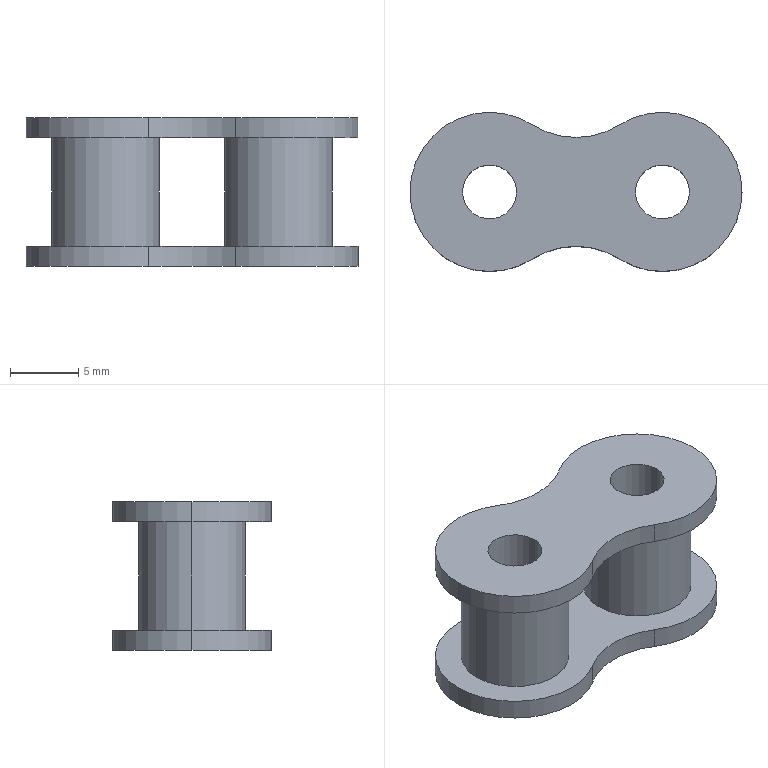Part | STEP file | _CHE40-500_c2 | 1 solid | 24 faces | box 24.4 x 11.7 x 10.95 mm | volume 1210 mm3 | cylinder 20 | plane 4 | commonest cylinder face diameters 11.7 x8 3.97 x4 7.92 x4 11.946 x4
STEP:
#1=CARTESIAN_POINT('',(3.142,4.935,-5.475));
#2=VERTEX_POINT('',#1);
#3=CARTESIAN_POINT('',(9.558,4.935,-5.475));
#4=VERTEX_POINT('',#3);
#5=CARTESIAN_POINT('',(6.35,9.973,-5.475));
#6=DIRECTION('',(0.,0.,1.));
#7=AXIS2_PLACEMENT_3D('',#5,#6,$);
#8=CIRCLE('',#7,5.973);
#9=EDGE_CURVE('',#2,#4,#8,.T.);
#10=ORIENTED_EDGE('',*,*,#9,.T.);
#11=CARTESIAN_POINT('',(18.55,0.,-5.475));
#12=VERTEX_POINT('',#11);
#13=CARTESIAN_POINT('',(12.7,0.,-5.475));
#14=DIRECTION('',(0.,0.,1.));
#15=AXIS2_PLACEMENT_3D('',#13,#14,$);
#16=CIRCLE('',#15,5.85);
#17=EDGE_CURVE('',#12,#4,#16,.T.);
#18=ORIENTED_EDGE('',*,*,#17,.F.);
#19=CARTESIAN_POINT('',(9.558,-4.935,-5.475));
#20=VERTEX_POINT('',#19);
#21=CARTESIAN_POINT('',(12.7,0.,-5.475));
#22=DIRECTION('',(0.,0.,1.));
#23=AXIS2_PLACEMENT_3D('',#21,#22,$);
#24=CIRCLE('',#23,5.85);
#25=EDGE_CURVE('',#20,#12,#24,.T.);
#26=ORIENTED_EDGE('',*,*,#25,.F.);
#27=CARTESIAN_POINT('',(3.142,-4.935,-5.475));
#28=VERTEX_POINT('',#27);
#29=CARTESIAN_POINT('',(6.35,-9.973,-5.475));
#30=DIRECTION('',(0.,0.,1.));
#31=AXIS2_PLACEMENT_3D('',#29,#30,$);
#32=CIRCLE('',#31,5.973);
#33=EDGE_CURVE('',#20,#28,#32,.T.);
#34=ORIENTED_EDGE('',*,*,#33,.T.);
#35=CARTESIAN_POINT('',(-5.85,0.,-5.475));
#36=VERTEX_POINT('',#35);
#37=CARTESIAN_POINT('',(0.,-0.000000001,-5.475));
#38=DIRECTION('',(0.,0.,1.));
#39=AXIS2_PLACEMENT_3D('',#37,#38,$);
#40=CIRCLE('',#39,5.85);
#41=EDGE_CURVE('',#36,#28,#40,.T.);
#42=ORIENTED_EDGE('',*,*,#41,.F.);
#43=CARTESIAN_POINT('',(0.,-0.000000001,-5.475));
#44=DIRECTION('',(0.,0.,1.));
#45=AXIS2_PLACEMENT_3D('',#43,#44,$);
#46=CIRCLE('',#45,5.85);
#47=EDGE_CURVE('',#2,#36,#46,.T.);
#48=ORIENTED_EDGE('',*,*,#47,.F.);
#49=EDGE_LOOP('',(#10,#18,#26,#34,#42,#48));
#50=FACE_OUTER_BOUND('',#49,.T.);
#51=CARTESIAN_POINT('',(10.715,0.000000001,-5.475));
#52=VERTEX_POINT('',#51);
#53=CARTESIAN_POINT('',(14.685,0.000000001,-5.475));
#54=VERTEX_POINT('',#53);
#55=CARTESIAN_POINT('',(12.7,0.,-5.475));
#56=DIRECTION('',(0.,0.,1.));
#57=AXIS2_PLACEMENT_3D('',#55,#56,$);
#58=CIRCLE('',#57,1.985);
#59=EDGE_CURVE('',#52,#54,#58,.F.);
#60=ORIENTED_EDGE('',*,*,#59,.F.);
#61=CARTESIAN_POINT('',(12.7,0.,-5.475));
#62=DIRECTION('',(0.,0.,1.));
#63=AXIS2_PLACEMENT_3D('',#61,#62,$);
#64=CIRCLE('',#63,1.985);
#65=EDGE_CURVE('',#54,#52,#64,.F.);
#66=ORIENTED_EDGE('',*,*,#65,.F.);
#67=EDGE_LOOP('',(#60,#66));
#68=FACE_BOUND('',#67,.T.);
#69=CARTESIAN_POINT('',(-1.985,0.000000001,-5.475));
#70=VERTEX_POINT('',#69);
#71=CARTESIAN_POINT('',(1.985,0.000000001,-5.475));
#72=VERTEX_POINT('',#71);
#73=CARTESIAN_POINT('',(0.000000001,0.,-5.475));
#74=DIRECTION('',(0.,0.,1.));
#75=AXIS2_PLACEMENT_3D('',#73,#74,$);
#76=CIRCLE('',#75,1.985);
#77=EDGE_CURVE('',#70,#72,#76,.F.);
#78=ORIENTED_EDGE('',*,*,#77,.F.);
#79=CARTESIAN_POINT('',(0.000000001,0.,-5.475));
#80=DIRECTION('',(0.,0.,1.));
#81=AXIS2_PLACEMENT_3D('',#79,#80,$);
#82=CIRCLE('',#81,1.985);
#83=EDGE_CURVE('',#72,#70,#82,.F.);
#84=ORIENTED_EDGE('',*,*,#83,.F.);
#85=EDGE_LOOP('',(#78,#84));
#86=FACE_BOUND('',#85,.T.);
#87=CARTESIAN_POINT('',(9.525,4.986,-5.475));
#88=DIRECTION('',(0.,0.,1.));
#89=DIRECTION('',(1.,0.,0.));
#90=AXIS2_PLACEMENT_3D('',#87,#88,#89);
#91=PLANE('',#90);
#92=ADVANCED_FACE('',(#50,#68,#86),#91,.F.);
#93=CARTESIAN_POINT('',(3.142,4.935,-3.975));
#94=VERTEX_POINT('',#93);
#95=CARTESIAN_POINT('',(9.558,4.935,-3.975));
#96=VERTEX_POINT('',#95);
#97=CARTESIAN_POINT('',(6.35,9.973,-3.975));
#98=DIRECTION('',(0.,0.,-1.));
#99=AXIS2_PLACEMENT_3D('',#97,#98,$);
#100=CIRCLE('',#99,5.973);
#101=EDGE_CURVE('',#94,#96,#100,.F.);
#102=ORIENTED_EDGE('',*,*,#101,.T.);
#103=CARTESIAN_POINT('',(9.558,4.935,-5.475));
#104=DIRECTION('',(0.,0.,-1.));
#105=VECTOR('',#104,1.);
#106=LINE('',#103,#105);
#107=EDGE_CURVE('',#4,#96,#106,.F.);
#108=ORIENTED_EDGE('',*,*,#107,.F.);
#109=ORIENTED_EDGE('',*,*,#9,.F.);
#110=CARTESIAN_POINT('',(3.142,4.935,-5.475));
#111=DIRECTION('',(0.,0.,-1.));
#112=VECTOR('',#111,1.);
#113=LINE('',#110,#112);
#114=EDGE_CURVE('',#2,#94,#113,.F.);
#115=ORIENTED_EDGE('',*,*,#114,.T.);
#116=EDGE_LOOP('',(#102,#108,#109,#115));
#117=FACE_OUTER_BOUND('',#116,.T.);
#118=CARTESIAN_POINT('',(6.35,9.973,-5.475));
#119=DIRECTION('',(0.,0.,-1.));
#120=DIRECTION('',(1.,0.,0.));
#121=AXIS2_PLACEMENT_3D('',#118,#119,#120);
#122=CYLINDRICAL_SURFACE('',#121,5.973);
#123=ADVANCED_FACE('',(#117),#122,.F.);
#124=CARTESIAN_POINT('',(18.55,0.,-3.975));
#125=VERTEX_POINT('',#124);
#126=CARTESIAN_POINT('',(18.55,0.,-5.475));
#127=DIRECTION('',(0.,0.,-1.));
#128=VECTOR('',#127,1.);
#129=LINE('',#126,#128);
#130=EDGE_CURVE('',#12,#125,#129,.F.);
#131=ORIENTED_EDGE('',*,*,#130,.F.);
#132=ORIENTED_EDGE('',*,*,#17,.T.);
#133=ORIENTED_EDGE('',*,*,#107,.T.);
#134=CARTESIAN_POINT('',(12.7,0.,-3.975));
#135=DIRECTION('',(0.,0.,-1.));
#136=AXIS2_PLACEMENT_3D('',#134,#135,$);
#137=CIRCLE('',#136,5.85);
#138=EDGE_CURVE('',#125,#96,#137,.F.);
#139=ORIENTED_EDGE('',*,*,#138,.F.);
#140=EDGE_LOOP('',(#131,#132,#133,#139));
#141=FACE_OUTER_BOUND('',#140,.T.);
#142=CARTESIAN_POINT('',(12.7,0.,-5.475));
#143=DIRECTION('',(0.,0.,-1.));
#144=DIRECTION('',(-1.,0.,0.));
#145=AXIS2_PLACEMENT_3D('',#142,#143,#144);
#146=CYLINDRICAL_SURFACE('',#145,5.85);
#147=ADVANCED_FACE('',(#141),#146,.T.);
#148=ORIENTED_EDGE('',*,*,#130,.T.);
#149=CARTESIAN_POINT('',(9.558,-4.935,-3.975));
#150=VERTEX_POINT('',#149);
#151=CARTESIAN_POINT('',(12.7,0.,-3.975));
#152=DIRECTION('',(0.,0.,-1.));
#153=AXIS2_PLACEMENT_3D('',#151,#152,$);
#154=CIRCLE('',#153,5.85);
#155=EDGE_CURVE('',#150,#125,#154,.F.);
#156=ORIENTED_EDGE('',*,*,#155,.F.);
#157=CARTESIAN_POINT('',(9.558,-4.935,-5.475));
#158=DIRECTION('',(0.,0.,-1.));
#159=VECTOR('',#158,1.);
#160=LINE('',#157,#159);
#161=EDGE_CURVE('',#20,#150,#160,.F.);
#162=ORIENTED_EDGE('',*,*,#161,.F.);
#163=ORIENTED_EDGE('',*,*,#25,.T.);
#164=EDGE_LOOP('',(#148,#156,#162,#163));
#165=FACE_OUTER_BOUND('',#164,.T.);
#166=CARTESIAN_POINT('',(12.7,0.,-5.475));
#167=DIRECTION('',(0.,0.,-1.));
#168=DIRECTION('',(1.,0.,0.));
#169=AXIS2_PLACEMENT_3D('',#166,#167,#168);
#170=CYLINDRICAL_SURFACE('',#169,5.85);
#171=ADVANCED_FACE('',(#165),#170,.T.);
#172=CARTESIAN_POINT('',(3.142,-4.935,-3.975));
#173=VERTEX_POINT('',#172);
#174=CARTESIAN_POINT('',(6.35,-9.973,-3.975));
#175=DIRECTION('',(0.,0.,-1.));
#176=AXIS2_PLACEMENT_3D('',#174,#175,$);
#177=CIRCLE('',#176,5.973);
#178=EDGE_CURVE('',#150,#173,#177,.F.);
#179=ORIENTED_EDGE('',*,*,#178,.T.);
#180=CARTESIAN_POINT('',(3.142,-4.935,-5.475));
#181=DIRECTION('',(0.,0.,-1.));
#182=VECTOR('',#181,1.);
#183=LINE('',#180,#182);
#184=EDGE_CURVE('',#28,#173,#183,.F.);
#185=ORIENTED_EDGE('',*,*,#184,.F.);
#186=ORIENTED_EDGE('',*,*,#33,.F.);
#187=ORIENTED_EDGE('',*,*,#161,.T.);
#188=EDGE_LOOP('',(#179,#185,#186,#187));
#189=FACE_OUTER_BOUND('',#188,.T.);
#190=CARTESIAN_POINT('',(6.35,-9.973,-5.475));
#191=DIRECTION('',(0.,0.,-1.));
#192=DIRECTION('',(-1.,0.,0.));
#193=AXIS2_PLACEMENT_3D('',#190,#191,#192);
#194=CYLINDRICAL_SURFACE('',#193,5.973);
#195=ADVANCED_FACE('',(#189),#194,.F.);
#196=CARTESIAN_POINT('',(-5.85,0.,-3.975));
#197=VERTEX_POINT('',#196);
#198=CARTESIAN_POINT('',(-5.85,0.,-5.475));
#199=DIRECTION('',(0.,0.,-1.));
#200=VECTOR('',#199,1.);
#201=LINE('',#198,#200);
#202=EDGE_CURVE('',#197,#36,#201,.T.);
#203=ORIENTED_EDGE('',*,*,#202,.T.);
#204=ORIENTED_EDGE('',*,*,#41,.T.);
#205=ORIENTED_EDGE('',*,*,#184,.T.);
#206=CARTESIAN_POINT('',(0.,0.,-3.975));
#207=DIRECTION('',(0.,0.,-1.));
#208=AXIS2_PLACEMENT_3D('',#206,#207,$);
#209=CIRCLE('',#208,5.85);
#210=EDGE_CURVE('',#197,#173,#209,.F.);
#211=ORIENTED_EDGE('',*,*,#210,.F.);
#212=EDGE_LOOP('',(#203,#204,#205,#211));
#213=FACE_OUTER_BOUND('',#212,.T.);
#214=CARTESIAN_POINT('',(0.,0.,-5.475));
#215=DIRECTION('',(0.,0.,-1.));
#216=DIRECTION('',(1.,0.,0.));
#217=AXIS2_PLACEMENT_3D('',#214,#215,#216);
#218=CYLINDRICAL_SURFACE('',#217,5.85);
#219=ADVANCED_FACE('',(#213),#218,.T.);
#220=ORIENTED_EDGE('',*,*,#202,.F.);
#221=CARTESIAN_POINT('',(0.,0.,-3.975));
#222=DIRECTION('',(0.,0.,-1.));
#223=AXIS2_PLACEMENT_3D('',#221,#222,$);
#224=CIRCLE('',#223,5.85);
#225=EDGE_CURVE('',#94,#197,#224,.F.);
#226=ORIENTED_EDGE('',*,*,#225,.F.);
#227=ORIENTED_EDGE('',*,*,#114,.F.);
#228=ORIENTED_EDGE('',*,*,#47,.T.);
#229=EDGE_LOOP('',(#220,#226,#227,#228));
#230=FACE_OUTER_BOUND('',#229,.T.);
#231=CARTESIAN_POINT('',(0.,0.,-5.475));
#232=DIRECTION('',(0.,0.,-1.));
#233=DIRECTION('',(-1.,0.,0.));
#234=AXIS2_PLACEMENT_3D('',#231,#232,#233);
#235=CYLINDRICAL_SURFACE('',#234,5.85);
#236=ADVANCED_FACE('',(#230),#235,.T.);
#237=CARTESIAN_POINT('',(10.715,0.000000001,5.475));
#238=VERTEX_POINT('',#237);
#239=CARTESIAN_POINT('',(14.685,0.000000001,5.475));
#240=VERTEX_POINT('',#239);
#241=CARTESIAN_POINT('',(12.7,0.,5.475));
#242=DIRECTION('',(0.,0.,-1.));
#243=AXIS2_PLACEMENT_3D('',#241,#242,$);
#244=CIRCLE('',#243,1.985);
#245=EDGE_CURVE('',#238,#240,#244,.T.);
#246=ORIENTED_EDGE('',*,*,#245,.F.);
#247=CARTESIAN_POINT('',(10.715,0.,6.975));
#248=DIRECTION('',(0.,0.,-1.));
#249=VECTOR('',#248,1.);
#250=LINE('',#247,#249);
#251=EDGE_CURVE('',#238,#52,#250,.T.);
#252=ORIENTED_EDGE('',*,*,#251,.T.);
#253=ORIENTED_EDGE('',*,*,#59,.T.);
#254=CARTESIAN_POINT('',(14.685,0.,6.975));
#255=DIRECTION('',(0.,0.,-1.));
#256=VECTOR('',#255,1.);
#257=LINE('',#254,#256);
#258=EDGE_CURVE('',#54,#240,#257,.F.);
#259=ORIENTED_EDGE('',*,*,#258,.T.);
#260=EDGE_LOOP('',(#246,#252,#253,#259));
#261=FACE_OUTER_BOUND('',#260,.T.);
#262=CARTESIAN_POINT('',(12.7,0.,6.975));
#263=DIRECTION('',(0.,0.,-1.));
#264=DIRECTION('',(-1.,0.,0.));
#265=AXIS2_PLACEMENT_3D('',#262,#263,#264);
#266=CYLINDRICAL_SURFACE('',#265,1.985);
#267=ADVANCED_FACE('',(#261),#266,.F.);
#268=CARTESIAN_POINT('',(12.7,0.,5.475));
#269=DIRECTION('',(0.,0.,-1.));
#270=AXIS2_PLACEMENT_3D('',#268,#269,$);
#271=CIRCLE('',#270,1.985);
#272=EDGE_CURVE('',#240,#238,#271,.T.);
#273=ORIENTED_EDGE('',*,*,#272,.F.);
#274=ORIENTED_EDGE('',*,*,#258,.F.);
#275=ORIENTED_EDGE('',*,*,#65,.T.);
#276=ORIENTED_EDGE('',*,*,#251,.F.);
#277=EDGE_LOOP('',(#273,#274,#275,#276));
#278=FACE_OUTER_BOUND('',#277,.T.);
#279=CARTESIAN_POINT('',(12.7,0.,6.975));
#280=DIRECTION('',(0.,0.,-1.));
#281=DIRECTION('',(1.,0.,0.));
#282=AXIS2_PLACEMENT_3D('',#279,#280,#281);
#283=CYLINDRICAL_SURFACE('',#282,1.985);
#284=ADVANCED_FACE('',(#278),#283,.F.);
#285=CARTESIAN_POINT('',(-1.985,0.000000001,5.475));
#286=VERTEX_POINT('',#285);
#287=CARTESIAN_POINT('',(1.985,0.000000001,5.475));
#288=VERTEX_POINT('',#287);
#289=CARTESIAN_POINT('',(0.,0.,5.475));
#290=DIRECTION('',(0.,0.,-1.));
#291=AXIS2_PLACEMENT_3D('',#289,#290,$);
#292=CIRCLE('',#291,1.985);
#293=EDGE_CURVE('',#286,#288,#292,.T.);
#294=ORIENTED_EDGE('',*,*,#293,.F.);
#295=CARTESIAN_POINT('',(-1.985,0.,6.975));
#296=DIRECTION('',(0.,0.,-1.));
#297=VECTOR('',#296,1.);
#298=LINE('',#295,#297);
#299=EDGE_CURVE('',#286,#70,#298,.T.);
#300=ORIENTED_EDGE('',*,*,#299,.T.);
#301=ORIENTED_EDGE('',*,*,#77,.T.);
#302=CARTESIAN_POINT('',(1.985,0.,6.975));
#303=DIRECTION('',(0.,0.,-1.));
#304=VECTOR('',#303,1.);
#305=LINE('',#302,#304);
#306=EDGE_CURVE('',#72,#288,#305,.F.);
#307=ORIENTED_EDGE('',*,*,#306,.T.);
#308=EDGE_LOOP('',(#294,#300,#301,#307));
#309=FACE_OUTER_BOUND('',#308,.T.);
#310=CARTESIAN_POINT('',(0.,0.,6.975));
#311=DIRECTION('',(0.,0.,-1.));
#312=DIRECTION('',(-1.,0.,0.));
#313=AXIS2_PLACEMENT_3D('',#310,#311,#312);
#314=CYLINDRICAL_SURFACE('',#313,1.985);
#315=ADVANCED_FACE('',(#309),#314,.F.);
#316=CARTESIAN_POINT('',(0.,0.,5.475));
#317=DIRECTION('',(0.,0.,-1.));
#318=AXIS2_PLACEMENT_3D('',#316,#317,$);
#319=CIRCLE('',#318,1.985);
#320=EDGE_CURVE('',#288,#286,#319,.T.);
#321=ORIENTED_EDGE('',*,*,#320,.F.);
#322=ORIENTED_EDGE('',*,*,#306,.F.);
#323=ORIENTED_EDGE('',*,*,#83,.T.);
#324=ORIENTED_EDGE('',*,*,#299,.F.);
#325=EDGE_LOOP('',(#321,#322,#323,#324));
#326=FACE_OUTER_BOUND('',#325,.T.);
#327=CARTESIAN_POINT('',(0.,0.,6.975));
#328=DIRECTION('',(0.,0.,-1.));
#329=DIRECTION('',(1.,0.,0.));
#330=AXIS2_PLACEMENT_3D('',#327,#328,#329);
#331=CYLINDRICAL_SURFACE('',#330,1.985);
#332=ADVANCED_FACE('',(#326),#331,.F.);
#333=ORIENTED_EDGE('',*,*,#101,.F.);
#334=ORIENTED_EDGE('',*,*,#225,.T.);
#335=ORIENTED_EDGE('',*,*,#210,.T.);
#336=ORIENTED_EDGE('',*,*,#178,.F.);
#337=ORIENTED_EDGE('',*,*,#155,.T.);
#338=ORIENTED_EDGE('',*,*,#138,.T.);
#339=EDGE_LOOP('',(#333,#334,#335,#336,#337,#338));
#340=FACE_OUTER_BOUND('',#339,.T.);
#341=CARTESIAN_POINT('',(-3.96,0.000000001,-3.975));
#342=VERTEX_POINT('',#341);
#343=CARTESIAN_POINT('',(3.96,0.000000001,-3.975));
#344=VERTEX_POINT('',#343);
#345=CARTESIAN_POINT('',(0.000000001,0.,-3.975));
#346=DIRECTION('',(0.,0.,1.));
#347=AXIS2_PLACEMENT_3D('',#345,#346,$);
#348=CIRCLE('',#347,3.96);
#349=EDGE_CURVE('',#342,#344,#348,.T.);
#350=ORIENTED_EDGE('',*,*,#349,.F.);
#351=CARTESIAN_POINT('',(0.000000001,0.,-3.975));
#352=DIRECTION('',(0.,0.,1.));
#353=AXIS2_PLACEMENT_3D('',#351,#352,$);
#354=CIRCLE('',#353,3.96);
#355=EDGE_CURVE('',#344,#342,#354,.T.);
#356=ORIENTED_EDGE('',*,*,#355,.F.);
#357=EDGE_LOOP('',(#350,#356));
#358=FACE_BOUND('',#357,.T.);
#359=CARTESIAN_POINT('',(8.74,0.000000001,-3.975));
#360=VERTEX_POINT('',#359);
#361=CARTESIAN_POINT('',(16.66,0.000000001,-3.975));
#362=VERTEX_POINT('',#361);
#363=CARTESIAN_POINT('',(12.7,0.,-3.975));
#364=DIRECTION('',(0.,0.,1.));
#365=AXIS2_PLACEMENT_3D('',#363,#364,$);
#366=CIRCLE('',#365,3.96);
#367=EDGE_CURVE('',#360,#362,#366,.T.);
#368=ORIENTED_EDGE('',*,*,#367,.F.);
#369=CARTESIAN_POINT('',(12.7,0.,-3.975));
#370=DIRECTION('',(0.,0.,1.));
#371=AXIS2_PLACEMENT_3D('',#369,#370,$);
#372=CIRCLE('',#371,3.96);
#373=EDGE_CURVE('',#362,#360,#372,.T.);
#374=ORIENTED_EDGE('',*,*,#373,.F.);
#375=EDGE_LOOP('',(#368,#374));
#376=FACE_BOUND('',#375,.T.);
#377=CARTESIAN_POINT('',(9.525,4.986,-3.975));
#378=DIRECTION('',(0.,0.,1.));
#379=DIRECTION('',(1.,0.,0.));
#380=AXIS2_PLACEMENT_3D('',#377,#378,#379);
#381=PLANE('',#380);
#382=ADVANCED_FACE('',(#340,#358,#376),#381,.T.);
#383=CARTESIAN_POINT('',(3.142,4.935,5.475));
#384=VERTEX_POINT('',#383);
#385=CARTESIAN_POINT('',(9.558,4.935,5.475));
#386=VERTEX_POINT('',#385);
#387=CARTESIAN_POINT('',(6.35,9.973,5.475));
#388=DIRECTION('',(0.,0.,1.));
#389=AXIS2_PLACEMENT_3D('',#387,#388,$);
#390=CIRCLE('',#389,5.973);
#391=EDGE_CURVE('',#384,#386,#390,.T.);
#392=ORIENTED_EDGE('',*,*,#391,.F.);
#393=CARTESIAN_POINT('',(-5.85,0.,5.475));
#394=VERTEX_POINT('',#393);
#395=CARTESIAN_POINT('',(0.,-0.000000001,5.475));
#396=DIRECTION('',(0.,0.,1.));
#397=AXIS2_PLACEMENT_3D('',#395,#396,$);
#398=CIRCLE('',#397,5.85);
#399=EDGE_CURVE('',#384,#394,#398,.T.);
#400=ORIENTED_EDGE('',*,*,#399,.T.);
#401=CARTESIAN_POINT('',(3.142,-4.935,5.475));
#402=VERTEX_POINT('',#401);
#403=CARTESIAN_POINT('',(0.,-0.000000001,5.475));
#404=DIRECTION('',(0.,0.,1.));
#405=AXIS2_PLACEMENT_3D('',#403,#404,$);
#406=CIRCLE('',#405,5.85);
#407=EDGE_CURVE('',#394,#402,#406,.T.);
#408=ORIENTED_EDGE('',*,*,#407,.T.);
#409=CARTESIAN_POINT('',(9.558,-4.935,5.475));
#410=VERTEX_POINT('',#409);
#411=CARTESIAN_POINT('',(6.35,-9.973,5.475));
#412=DIRECTION('',(0.,0.,1.));
#413=AXIS2_PLACEMENT_3D('',#411,#412,$);
#414=CIRCLE('',#413,5.973);
#415=EDGE_CURVE('',#410,#402,#414,.T.);
#416=ORIENTED_EDGE('',*,*,#415,.F.);
#417=CARTESIAN_POINT('',(18.55,0.,5.475));
#418=VERTEX_POINT('',#417);
#419=CARTESIAN_POINT('',(12.7,0.,5.475));
#420=DIRECTION('',(0.,0.,1.));
#421=AXIS2_PLACEMENT_3D('',#419,#420,$);
#422=CIRCLE('',#421,5.85);
#423=EDGE_CURVE('',#410,#418,#422,.T.);
#424=ORIENTED_EDGE('',*,*,#423,.T.);
#425=CARTESIAN_POINT('',(12.7,0.,5.475));
#426=DIRECTION('',(0.,0.,1.));
#427=AXIS2_PLACEMENT_3D('',#425,#426,$);
#428=CIRCLE('',#427,5.85);
#429=EDGE_CURVE('',#418,#386,#428,.T.);
#430=ORIENTED_EDGE('',*,*,#429,.T.);
#431=EDGE_LOOP('',(#392,#400,#408,#416,#424,#430));
#432=FACE_OUTER_BOUND('',#431,.T.);
#433=ORIENTED_EDGE('',*,*,#272,.T.);
#434=ORIENTED_EDGE('',*,*,#245,.T.);
#435=EDGE_LOOP('',(#433,#434));
#436=FACE_BOUND('',#435,.T.);
#437=ORIENTED_EDGE('',*,*,#320,.T.);
#438=ORIENTED_EDGE('',*,*,#293,.T.);
#439=EDGE_LOOP('',(#437,#438));
#440=FACE_BOUND('',#439,.T.);
#441=CARTESIAN_POINT('',(9.525,4.986,5.475));
#442=DIRECTION('',(0.,0.,1.));
#443=DIRECTION('',(1.,0.,0.));
#444=AXIS2_PLACEMENT_3D('',#441,#442,#443);
#445=PLANE('',#444);
#446=ADVANCED_FACE('',(#432,#436,#440),#445,.T.);
#447=CARTESIAN_POINT('',(-3.96,0.000000001,3.975));
#448=VERTEX_POINT('',#447);
#449=CARTESIAN_POINT('',(-3.96,0.,4.725));
#450=DIRECTION('',(0.,0.,-1.));
#451=VECTOR('',#450,1.);
#452=LINE('',#449,#451);
#453=EDGE_CURVE('',#448,#342,#452,.T.);
#454=ORIENTED_EDGE('',*,*,#453,.T.);
#455=ORIENTED_EDGE('',*,*,#349,.T.);
#456=CARTESIAN_POINT('',(3.96,0.000000001,3.975));
#457=VERTEX_POINT('',#456);
#458=CARTESIAN_POINT('',(3.96,0.,4.725));
#459=DIRECTION('',(0.,0.,-1.));
#460=VECTOR('',#459,1.);
#461=LINE('',#458,#460);
#462=EDGE_CURVE('',#344,#457,#461,.F.);
#463=ORIENTED_EDGE('',*,*,#462,.T.);
#464=CARTESIAN_POINT('',(0.,0.,3.975));
#465=DIRECTION('',(0.,0.,-1.));
#466=AXIS2_PLACEMENT_3D('',#464,#465,$);
#467=CIRCLE('',#466,3.96);
#468=EDGE_CURVE('',#457,#448,#467,.T.);
#469=ORIENTED_EDGE('',*,*,#468,.T.);
#470=EDGE_LOOP('',(#454,#455,#463,#469));
#471=FACE_OUTER_BOUND('',#470,.T.);
#472=CARTESIAN_POINT('',(0.,0.,4.725));
#473=DIRECTION('',(0.,0.,-1.));
#474=DIRECTION('',(1.,0.,0.));
#475=AXIS2_PLACEMENT_3D('',#472,#473,#474);
#476=CYLINDRICAL_SURFACE('',#475,3.96);
#477=ADVANCED_FACE('',(#471),#476,.T.);
#478=ORIENTED_EDGE('',*,*,#462,.F.);
#479=ORIENTED_EDGE('',*,*,#355,.T.);
#480=ORIENTED_EDGE('',*,*,#453,.F.);
#481=CARTESIAN_POINT('',(0.,0.,3.975));
#482=DIRECTION('',(0.,0.,-1.));
#483=AXIS2_PLACEMENT_3D('',#481,#482,$);
#484=CIRCLE('',#483,3.96);
#485=EDGE_CURVE('',#448,#457,#484,.T.);
#486=ORIENTED_EDGE('',*,*,#485,.T.);
#487=EDGE_LOOP('',(#478,#479,#480,#486));
#488=FACE_OUTER_BOUND('',#487,.T.);
#489=CARTESIAN_POINT('',(0.,0.,4.725));
#490=DIRECTION('',(0.,0.,-1.));
#491=DIRECTION('',(-1.,0.,0.));
#492=AXIS2_PLACEMENT_3D('',#489,#490,#491);
#493=CYLINDRICAL_SURFACE('',#492,3.96);
#494=ADVANCED_FACE('',(#488),#493,.T.);
#495=CARTESIAN_POINT('',(8.74,0.000000001,3.975));
#496=VERTEX_POINT('',#495);
#497=CARTESIAN_POINT('',(8.74,0.,4.725));
#498=DIRECTION('',(0.,0.,-1.));
#499=VECTOR('',#498,1.);
#500=LINE('',#497,#499);
#501=EDGE_CURVE('',#496,#360,#500,.T.);
#502=ORIENTED_EDGE('',*,*,#501,.T.);
#503=ORIENTED_EDGE('',*,*,#367,.T.);
#504=CARTESIAN_POINT('',(16.66,0.000000001,3.975));
#505=VERTEX_POINT('',#504);
#506=CARTESIAN_POINT('',(16.66,0.,4.725));
#507=DIRECTION('',(0.,0.,-1.));
#508=VECTOR('',#507,1.);
#509=LINE('',#506,#508);
#510=EDGE_CURVE('',#362,#505,#509,.F.);
#511=ORIENTED_EDGE('',*,*,#510,.T.);
#512=CARTESIAN_POINT('',(12.7,0.,3.975));
#513=DIRECTION('',(0.,0.,-1.));
#514=AXIS2_PLACEMENT_3D('',#512,#513,$);
#515=CIRCLE('',#514,3.96);
#516=EDGE_CURVE('',#505,#496,#515,.T.);
#517=ORIENTED_EDGE('',*,*,#516,.T.);
#518=EDGE_LOOP('',(#502,#503,#511,#517));
#519=FACE_OUTER_BOUND('',#518,.T.);
#520=CARTESIAN_POINT('',(12.7,0.,4.725));
#521=DIRECTION('',(0.,0.,-1.));
#522=DIRECTION('',(1.,0.,0.));
#523=AXIS2_PLACEMENT_3D('',#520,#521,#522);
#524=CYLINDRICAL_SURFACE('',#523,3.96);
#525=ADVANCED_FACE('',(#519),#524,.T.);
#526=ORIENTED_EDGE('',*,*,#510,.F.);
#527=ORIENTED_EDGE('',*,*,#373,.T.);
#528=ORIENTED_EDGE('',*,*,#501,.F.);
#529=CARTESIAN_POINT('',(12.7,0.,3.975));
#530=DIRECTION('',(0.,0.,-1.));
#531=AXIS2_PLACEMENT_3D('',#529,#530,$);
#532=CIRCLE('',#531,3.96);
#533=EDGE_CURVE('',#496,#505,#532,.T.);
#534=ORIENTED_EDGE('',*,*,#533,.T.);
#535=EDGE_LOOP('',(#526,#527,#528,#534));
#536=FACE_OUTER_BOUND('',#535,.T.);
#537=CARTESIAN_POINT('',(12.7,0.,4.725));
#538=DIRECTION('',(0.,0.,-1.));
#539=DIRECTION('',(-1.,0.,0.));
#540=AXIS2_PLACEMENT_3D('',#537,#538,#539);
#541=CYLINDRICAL_SURFACE('',#540,3.96);
#542=ADVANCED_FACE('',(#536),#541,.T.);
#543=CARTESIAN_POINT('',(3.142,4.935,3.975));
#544=VERTEX_POINT('',#543);
#545=CARTESIAN_POINT('',(9.558,4.935,3.975));
#546=VERTEX_POINT('',#545);
#547=CARTESIAN_POINT('',(6.35,9.973,3.975));
#548=DIRECTION('',(0.,0.,1.));
#549=AXIS2_PLACEMENT_3D('',#547,#548,$);
#550=CIRCLE('',#549,5.973);
#551=EDGE_CURVE('',#544,#546,#550,.T.);
#552=ORIENTED_EDGE('',*,*,#551,.F.);
#553=CARTESIAN_POINT('',(3.142,4.935,5.475));
#554=DIRECTION('',(0.,0.,1.));
#555=VECTOR('',#554,1.);
#556=LINE('',#553,#555);
#557=EDGE_CURVE('',#384,#544,#556,.F.);
#558=ORIENTED_EDGE('',*,*,#557,.F.);
#559=ORIENTED_EDGE('',*,*,#391,.T.);
#560=CARTESIAN_POINT('',(9.558,4.935,5.475));
#561=DIRECTION('',(0.,0.,1.));
#562=VECTOR('',#561,1.);
#563=LINE('',#560,#562);
#564=EDGE_CURVE('',#386,#546,#563,.F.);
#565=ORIENTED_EDGE('',*,*,#564,.T.);
#566=EDGE_LOOP('',(#552,#558,#559,#565));
#567=FACE_OUTER_BOUND('',#566,.T.);
#568=CARTESIAN_POINT('',(6.35,9.973,5.475));
#569=DIRECTION('',(0.,0.,1.));
#570=DIRECTION('',(-1.,0.,0.));
#571=AXIS2_PLACEMENT_3D('',#568,#569,#570);
#572=CYLINDRICAL_SURFACE('',#571,5.973);
#573=ADVANCED_FACE('',(#567),#572,.F.);
#574=CARTESIAN_POINT('',(-5.85,0.,3.975));
#575=VERTEX_POINT('',#574);
#576=CARTESIAN_POINT('',(-5.85,0.,5.475));
#577=DIRECTION('',(0.,0.,1.));
#578=VECTOR('',#577,1.);
#579=LINE('',#576,#578);
#580=EDGE_CURVE('',#394,#575,#579,.F.);
#581=ORIENTED_EDGE('',*,*,#580,.F.);
#582=ORIENTED_EDGE('',*,*,#399,.F.);
#583=ORIENTED_EDGE('',*,*,#557,.T.);
#584=CARTESIAN_POINT('',(0.,0.,3.975));
#585=DIRECTION('',(0.,0.,1.));
#586=AXIS2_PLACEMENT_3D('',#584,#585,$);
#587=CIRCLE('',#586,5.85);
#588=EDGE_CURVE('',#544,#575,#587,.T.);
#589=ORIENTED_EDGE('',*,*,#588,.T.);
#590=EDGE_LOOP('',(#581,#582,#583,#589));
#591=FACE_OUTER_BOUND('',#590,.T.);
#592=CARTESIAN_POINT('',(0.,0.,5.475));
#593=DIRECTION('',(0.,0.,1.));
#594=DIRECTION('',(1.,0.,0.));
#595=AXIS2_PLACEMENT_3D('',#592,#593,#594);
#596=CYLINDRICAL_SURFACE('',#595,5.85);
#597=ADVANCED_FACE('',(#591),#596,.T.);
#598=ORIENTED_EDGE('',*,*,#580,.T.);
#599=CARTESIAN_POINT('',(3.142,-4.935,3.975));
#600=VERTEX_POINT('',#599);
#601=CARTESIAN_POINT('',(0.,0.,3.975));
#602=DIRECTION('',(0.,0.,1.));
#603=AXIS2_PLACEMENT_3D('',#601,#602,$);
#604=CIRCLE('',#603,5.85);
#605=EDGE_CURVE('',#575,#600,#604,.T.);
#606=ORIENTED_EDGE('',*,*,#605,.T.);
#607=CARTESIAN_POINT('',(3.142,-4.935,5.475));
#608=DIRECTION('',(0.,0.,1.));
#609=VECTOR('',#608,1.);
#610=LINE('',#607,#609);
#611=EDGE_CURVE('',#402,#600,#610,.F.);
#612=ORIENTED_EDGE('',*,*,#611,.F.);
#613=ORIENTED_EDGE('',*,*,#407,.F.);
#614=EDGE_LOOP('',(#598,#606,#612,#613));
#615=FACE_OUTER_BOUND('',#614,.T.);
#616=CARTESIAN_POINT('',(0.,0.,5.475));
#617=DIRECTION('',(0.,0.,1.));
#618=DIRECTION('',(-1.,0.,0.));
#619=AXIS2_PLACEMENT_3D('',#616,#617,#618);
#620=CYLINDRICAL_SURFACE('',#619,5.85);
#621=ADVANCED_FACE('',(#615),#620,.T.);
#622=CARTESIAN_POINT('',(9.558,-4.935,3.975));
#623=VERTEX_POINT('',#622);
#624=CARTESIAN_POINT('',(6.35,-9.973,3.975));
#625=DIRECTION('',(0.,0.,1.));
#626=AXIS2_PLACEMENT_3D('',#624,#625,$);
#627=CIRCLE('',#626,5.973);
#628=EDGE_CURVE('',#623,#600,#627,.T.);
#629=ORIENTED_EDGE('',*,*,#628,.F.);
#630=CARTESIAN_POINT('',(9.558,-4.935,5.475));
#631=DIRECTION('',(0.,0.,1.));
#632=VECTOR('',#631,1.);
#633=LINE('',#630,#632);
#634=EDGE_CURVE('',#410,#623,#633,.F.);
#635=ORIENTED_EDGE('',*,*,#634,.F.);
#636=ORIENTED_EDGE('',*,*,#415,.T.);
#637=ORIENTED_EDGE('',*,*,#611,.T.);
#638=EDGE_LOOP('',(#629,#635,#636,#637));
#639=FACE_OUTER_BOUND('',#638,.T.);
#640=CARTESIAN_POINT('',(6.35,-9.973,5.475));
#641=DIRECTION('',(0.,0.,1.));
#642=DIRECTION('',(1.,0.,0.));
#643=AXIS2_PLACEMENT_3D('',#640,#641,#642);
#644=CYLINDRICAL_SURFACE('',#643,5.973);
#645=ADVANCED_FACE('',(#639),#644,.F.);
#646=CARTESIAN_POINT('',(18.55,0.,3.975));
#647=VERTEX_POINT('',#646);
#648=CARTESIAN_POINT('',(18.55,0.,5.475));
#649=DIRECTION('',(0.,0.,1.));
#650=VECTOR('',#649,1.);
#651=LINE('',#648,#650);
#652=EDGE_CURVE('',#647,#418,#651,.T.);
#653=ORIENTED_EDGE('',*,*,#652,.T.);
#654=ORIENTED_EDGE('',*,*,#423,.F.);
#655=ORIENTED_EDGE('',*,*,#634,.T.);
#656=CARTESIAN_POINT('',(12.7,0.,3.975));
#657=DIRECTION('',(0.,0.,1.));
#658=AXIS2_PLACEMENT_3D('',#656,#657,$);
#659=CIRCLE('',#658,5.85);
#660=EDGE_CURVE('',#623,#647,#659,.T.);
#661=ORIENTED_EDGE('',*,*,#660,.T.);
#662=EDGE_LOOP('',(#653,#654,#655,#661));
#663=FACE_OUTER_BOUND('',#662,.T.);
#664=CARTESIAN_POINT('',(12.7,0.,5.475));
#665=DIRECTION('',(0.,0.,1.));
#666=DIRECTION('',(-1.,0.,0.));
#667=AXIS2_PLACEMENT_3D('',#664,#665,#666);
#668=CYLINDRICAL_SURFACE('',#667,5.85);
#669=ADVANCED_FACE('',(#663),#668,.T.);
#670=ORIENTED_EDGE('',*,*,#652,.F.);
#671=CARTESIAN_POINT('',(12.7,0.,3.975));
#672=DIRECTION('',(0.,0.,1.));
#673=AXIS2_PLACEMENT_3D('',#671,#672,$);
#674=CIRCLE('',#673,5.85);
#675=EDGE_CURVE('',#647,#546,#674,.T.);
#676=ORIENTED_EDGE('',*,*,#675,.T.);
#677=ORIENTED_EDGE('',*,*,#564,.F.);
#678=ORIENTED_EDGE('',*,*,#429,.F.);
#679=EDGE_LOOP('',(#670,#676,#677,#678));
#680=FACE_OUTER_BOUND('',#679,.T.);
#681=CARTESIAN_POINT('',(12.7,0.,5.475));
#682=DIRECTION('',(0.,0.,1.));
#683=DIRECTION('',(1.,0.,0.));
#684=AXIS2_PLACEMENT_3D('',#681,#682,#683);
#685=CYLINDRICAL_SURFACE('',#684,5.85);
#686=ADVANCED_FACE('',(#680),#685,.T.);
#687=ORIENTED_EDGE('',*,*,#551,.T.);
#688=ORIENTED_EDGE('',*,*,#675,.F.);
#689=ORIENTED_EDGE('',*,*,#660,.F.);
#690=ORIENTED_EDGE('',*,*,#628,.T.);
#691=ORIENTED_EDGE('',*,*,#605,.F.);
#692=ORIENTED_EDGE('',*,*,#588,.F.);
#693=EDGE_LOOP('',(#687,#688,#689,#690,#691,#692));
#694=FACE_OUTER_BOUND('',#693,.T.);
#695=ORIENTED_EDGE('',*,*,#533,.F.);
#696=ORIENTED_EDGE('',*,*,#516,.F.);
#697=EDGE_LOOP('',(#695,#696));
#698=FACE_BOUND('',#697,.T.);
#699=ORIENTED_EDGE('',*,*,#485,.F.);
#700=ORIENTED_EDGE('',*,*,#468,.F.);
#701=EDGE_LOOP('',(#699,#700));
#702=FACE_BOUND('',#701,.T.);
#703=CARTESIAN_POINT('',(9.525,4.986,3.975));
#704=DIRECTION('',(0.,0.,1.));
#705=DIRECTION('',(1.,0.,0.));
#706=AXIS2_PLACEMENT_3D('',#703,#704,#705);
#707=PLANE('',#706);
#708=ADVANCED_FACE('',(#694,#698,#702),#707,.F.);
#709=CLOSED_SHELL('',(#92,#123,#147,#171,#195,#219,#236,#267,#284,#315,#332,#382,#446,#477,#494,#525,#542,#573,#597,#621,#645,#669,#686,#708));
#710=MANIFOLD_SOLID_BREP('',#709);
#711=(LENGTH_UNIT()NAMED_UNIT(*)SI_UNIT(.MILLI.,.METRE.));
#712=UNCERTAINTY_MEASURE_WITH_UNIT(LENGTH_MEASURE(0.005),#711,'','');
#713=(NAMED_UNIT(*)PLANE_ANGLE_UNIT()SI_UNIT($,.RADIAN.));
#714=(NAMED_UNIT(*)SI_UNIT($,.STERADIAN.)SOLID_ANGLE_UNIT());
#715=(GEOMETRIC_REPRESENTATION_CONTEXT(3)GLOBAL_UNCERTAINTY_ASSIGNED_CONTEXT((#712))GLOBAL_UNIT_ASSIGNED_CONTEXT((#711,#713,#714))REPRESENTATION_CONTEXT('',''));
#716=ADVANCED_BREP_SHAPE_REPRESENTATION('',(#710),#715);